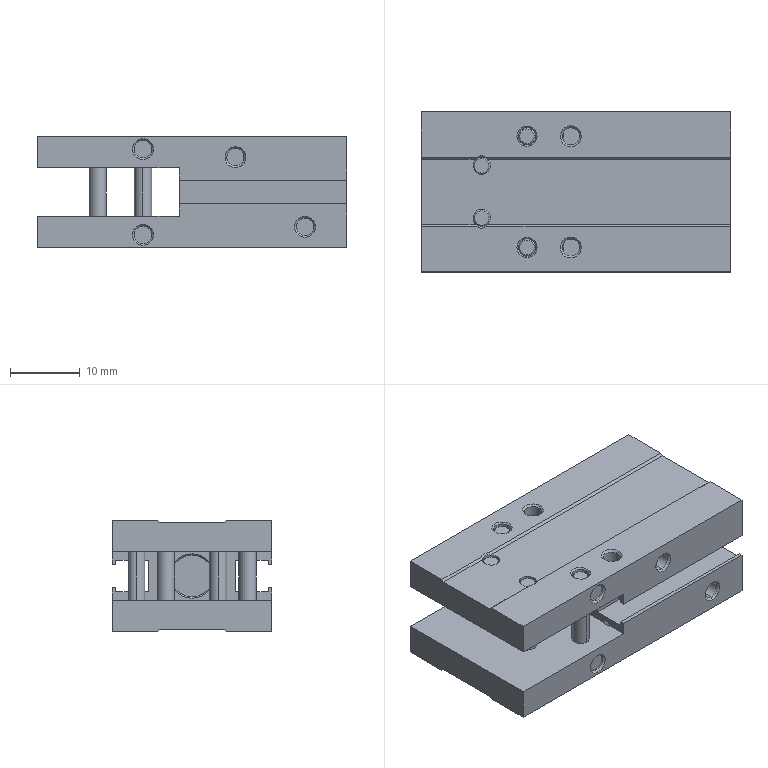Part | SolidWorks | features BaseBody 1 | 1 solid | 190 faces | box 44.5 x 23 x 16 mm | volume 10279 mm3 | plane 66 | cylinder 64 | cone 60 | commonest cylinder face diameters 2.5 x32 2.459 x16 2 x4 4.134 x4 6 x2 8 x2